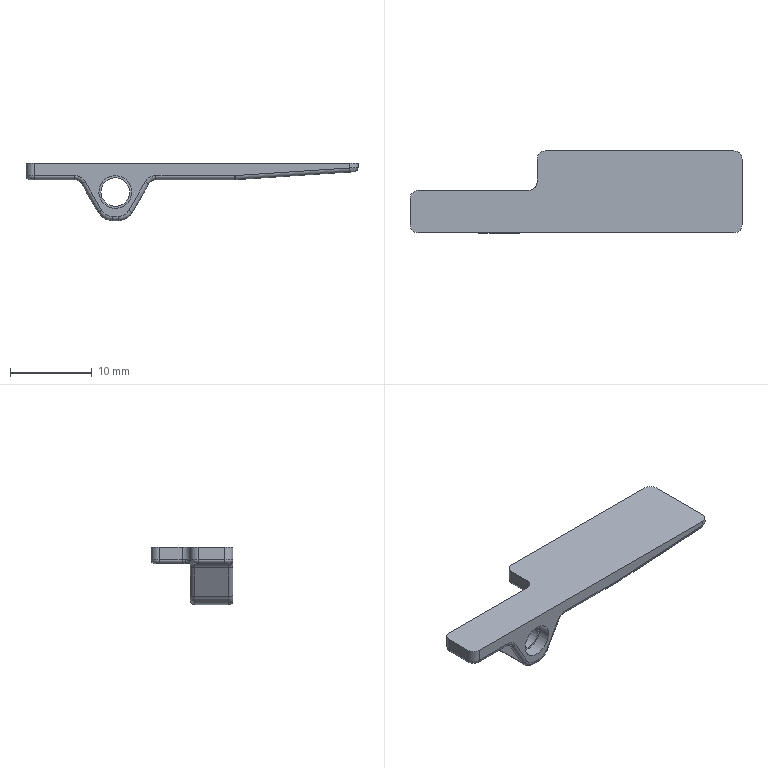NC program | Mastercam | posted with a generic post | part box 40.5 x 10 x 7 mm
Lines 1264 to 2237 of 12178:
(6 FEM |TOOL - 6|DIA. OFF. - 6|LEN. - 6|TOOL DIA. - 6.)
N2590 T6 M6
N2592 G0 G54 G90 X4.981 Y-3.575 C0. B0. S7000 M3
N2594 G43 H6 Z50.
N2596 Z.91
N2598 G1 Z.41 F600.
N2600 G2 X6.981 Y-1.582 Z.3 I2. J-.007 F2000.
N2602 G1 X6.987
N2604 X10.287 Y-1.592 Z.272
N2606 X13.587 Y-1.603 Z.243
N2608 X16.864 Y-1.614 Z.215
N2610 Y-1.212
N2612 Y1.614 Z.191
N2614 X15.161 Z.187
N2616 X11.861 Z.159
N2618 X8.561 Z.13
N2620 X7.761 Z.124
N2622 X5.261 Z.102
N2624 X1.961 Z.074
N2626 X-1.335 Z.046
N2628 G2 X-1.321 Y1.264 I-11.47 J-.649
N2630 G1 X-1.317 Y.965 Z.043
N2632 G2 X-1.596 Y-1.553 Z.021 I-11.488
N2634 G1 X.387 Y-1.56 Z.017
N2636 X3.258 Y-1.569 Z-.007
N2638 X3.687 Y-1.571 Z-.011
N2640 X6.987 Y-1.582 Z-.039
N2642 X10.287 Y-1.592 Z-.067
N2644 X13.587 Y-1.603 Z-.096
N2646 X16.864 Y-1.614 Z-.124
N2648 Y-1.217
N2650 Y1.614 Z-.148
N2652 X15.169 Z-.152
N2654 X11.869 Z-.18
N2656 X8.569 Z-.209
N2658 X7.761 Z-.216
N2660 X5.269 Z-.237
N2662 X1.969 Z-.265
N2664 X-1.335 Z-.293
N2666 G2 X-1.328 Y1.481 I-11.47 J-.649
N2668 X-1.316 Y.965 Z-.298 I-11.477 J-.516
N2670 X-1.596 Y-1.553 Z-.32 I-11.489
N2672 G1 X-.042 Y-1.558 Z-.322
N2674 X3.258 Y-1.569 Z-.35
N2676 X16.864 Y-1.614
N2678 Y1.614
N2680 X7.761
N2682 X-1.335
N2684 G2 X-1.317 Y.965 I-11.47 J-.649
N2686 X-1.596 Y-1.553 I-11.488
N2688 G1 X3.258 Y-1.569
N2690 G2 X3.78 Y-1.992 I-.002 J-.537
N2692 G1 X4.343 Y-4.578
N2694 G3 X4.867 Y-5. I.524 J.114
N2696 G1 X19.151
N2698 G3 X19.235 Y-5.003 I.084 J1.008
N2700 X20.241 Y-4.101 J1.011
N2702 G1 X20.25 Y3.944
N2704 G3 X20.251 Y3.992 I-1.004 J.048
N2706 X19.335 Y4.993 I-1.005
N2708 G1 X7.761 Y5.
N2710 X-4.762
N2712 X-4.721 Y4.463
N2714 X-4.723 Y.245
N2716 G2 X-4.78 Y-.299 I-2.999 J.042
N2718 G1 X-4.829 Y-.528
N2720 G2 X-5.27 Y-1.54 I-2.923 J.674
N2722 G1 X-5.281 Y-1.555
N2724 G2 X-4.75 Y-3.258 I-2.469 J-1.704
N2726 G1 Y-3.944
N2728 G3 X-4.751 Y-3.991 I1.004 J-.047
N2730 X-3.828 Y-4.993 I1.005
N2732 G1 X-3.635 Y-5.
N2734 X4.867
N2736 G3 X5.403 Y-4.464 J.536
N2738 X5.199 Y-4.043 I-.536
N2740 G1 X3.402 Y-2.622
N2742 G2 X3.198 Y-2.201 I.333 J.421
N2744 X3.735 Y-1.665 I.537
N2746 G1 X6.475 Z-.372
N2748 X7.035 Z-.377
N2750 X10.335 Z-.404
N2752 X13.635 Z-.431
N2754 X16.915 Z-.458
N2756 Y-1.302
N2758 Y1.665 Z-.482
N2760 X15.469 Z-.485
N2762 X12.169 Z-.512
N2764 X8.869 Z-.538
N2766 X7.937 Z-.546
N2768 X5.569 Z-.565
N2770 X2.269 Z-.592
N2772 X-1.035 Z-.619
N2774 G2 X-1.028 Y1.509 I-11.533 J-.653
N2776 G1 X-1.02 Y1.261 Z-.621
N2778 X-1.017 Y1.012 Z-.623
N2780 G2 X-1.331 Y-1.665 Z-.645 I-11.551
N2782 G1 X-.125 Z-.646
N2784 X3.175 Z-.673
N2786 X6.475 Z-.7
N2788 X16.915
N2790 Y1.665
N2792 X7.937
N2794 X-1.035
N2796 G2 X-1.017 Y1.012 I-11.533 J-.653
N2798 X-1.331 Y-1.665 I-11.551
N2800 G1 X6.475
N2802 G2 X6.999 Y-2.083 J-.536
N2804 G1 X7.561 Y-4.582
N2806 G3 X8.084 Y-5. I.523 J.118
N2808 G1 X19.151
N2810 G3 X19.235 Y-5.003 I.084 J1.008
N2812 X20.241 Y-4.101 J1.011
N2814 G1 X20.25 Y3.944
N2816 G3 X20.251 Y3.992 I-1.004 J.048
N2818 X19.335 Y4.993 I-1.005
N2820 G1 X7.937 Y5.
N2822 X-4.411
N2824 X-4.371 Y4.511
N2826 Y.383
N2828 X-4.372 Y.252
N2830 G2 X-4.416 Y-.229 I-3. J.035
N2832 X-5.11 Y-1.834 I-3.528 J.571
N2834 X-4.75 Y-3.258 I-2.64 J-1.425
N2836 G1 Y-3.944
N2838 G3 X-4.751 Y-3.991 I1.004 J-.047
N2840 X-3.828 Y-4.993 I1.005
N2842 G1 X-3.635 Y-5.
N2844 X8.084
N2846 G3 X8.62 Y-4.464 J.536
N2848 X8.428 Y-4.052 I-.536
N2850 G1 X6.831 Y-2.72
N2852 G2 X6.638 Y-2.308 I.343 J.412
N2854 X7.174 Y-1.772 I.536
N2856 G1 X9.693 Z-.721
N2858 X10.474 Z-.727
N2860 X13.774 Z-.754
N2862 X17.022 Z-.78
N2864 Y-1.185 Z-.781
N2866 Y1.772 Z-.805
N2868 X15.558 Z-.808
N2870 X12.258 Z-.835
N2872 X8.958 Z-.862
N2874 X8.051 Z-.869
N2876 X5.658 Z-.888
N2878 X2.358 Z-.915
N2880 X-.913 Z-.942
N2882 X-.926 Y1.449
N2884 G2 X-1.24 Y-1.772 Z-.969 I-31.263 J1.417
N2886 G1 X-.207
N2888 X3.093 Z-.996
N2890 X6.393 Z-1.023
N2892 X9.693 Z-1.05
N2894 X17.022
N2896 Y1.772
N2898 X8.051
N2900 X-.913
N2902 G2 X-1.24 Y-1.772 I-31.276 J1.094
N2904 G1 X9.693
N2906 G2 X10.215 Y-2.185 J-.536
N2908 G1 X10.78 Y-4.587
N2910 G3 X11.302 Y-5. I.522 J.123
N2912 G1 X19.151
N2914 G3 X19.235 Y-5.003 I.084 J1.008
N2916 X20.241 Y-4.101 J1.011
N2918 G1 X20.25 Y3.944
N2920 G3 X20.251 Y3.992 I-1.004 J.048
N2922 X19.335 Y4.993 I-1.005
N2924 G1 X8.051 Y5.
N2926 X-4.182
N2928 X-4.142 Y4.48
N2930 Y.353
N2932 X-4.178 Y-.175
N2934 X-4.2 Y-.312
N2936 G2 X-4.386 Y-.983 I-2.964 J.463
N2938 G1 X-4.478 Y-1.193
N2940 G2 X-5.017 Y-2.022 I-3.431 J1.64
N2942 X-4.75 Y-3.258 I-2.733 J-1.237
N2944 G1 Y-3.944
N2946 G3 X-4.751 Y-3.991 I1.004 J-.047
N2948 X-3.828 Y-4.993 I1.005
N2950 G1 X-3.635 Y-5.
N2952 X11.302
N2954 G3 X11.838 Y-4.464 J.536
N2956 X11.66 Y-4.064 I-.536
N2958 G1 X10.252 Y-2.802
N2960 G2 X10.074 Y-2.403 I.358 J.399
N2962 X10.61 Y-1.867 I.536
N2964 G1 X12.91 Z-1.069
N2966 X13.91 Z-1.077
N2968 X17.117 Z-1.103
N2970 Y-1.089 Z-1.104
N2972 Y1.867 Z-1.128
N2974 X15.65 Z-1.131
N2976 X12.35 Z-1.158
N2978 X9.05 Z-1.185
N2980 X8.152 Z-1.192
N2982 X5.75 Z-1.212
N2984 X2.45 Z-1.238
N2986 X-.808 Z-1.265
N2988 X-.816 Y1.391
N2990 G2 X-1.171 Y-1.867 Z-1.292 I-20.708 J.606
N2992 G1 X-.29
N2994 X3.01 Z-1.319
N2996 X6.31 Z-1.346
N2998 X9.61 Z-1.373
N3000 X12.91 Z-1.4
N3002 X17.117
N3004 Y1.867
N3006 X8.152
N3008 X-.808
N3010 G2 X-1.171 Y-1.867 I-20.716 J.13
N3012 G1 X12.91
N3014 G2 X13.431 Y-2.276 J-.536
N3016 G1 X13.998 Y-4.591
N3018 G3 X14.519 Y-5. I.521 J.127
N3020 G1 X19.151
N3022 G3 X19.235 Y-5.003 I.084 J1.008
N3024 X20.241 Y-4.101 J1.011
N3026 G1 X20.25 Y3.944
N3028 G3 X20.251 Y3.992 I-1.004 J.048
N3030 X19.335 Y4.993 I-1.005
N3032 G1 X8.152 Y5.
N3034 X-3.981
N3036 X-3.941 Y4.51
N3038 Y.353
N3040 X-3.98 Y-.191
N3042 X-4.018 Y-.413
N3044 G2 X-4.234 Y-1.1 I-2.949 J.551
N3046 G1 X-4.255 Y-1.147
N3048 G2 X-4.953 Y-2.175 I-3.579 J1.678
N3050 X-4.75 Y-3.258 I-2.797 J-1.084
N3052 G1 Y-3.944
N3054 G3 X-4.751 Y-3.991 I1.004 J-.047
N3056 X-3.828 Y-4.993 I1.005
N3058 G1 X-3.635 Y-5.
N3060 X14.519
N3062 G3 X15.055 Y-4.464 J.536
N3064 X14.892 Y-4.079 I-.536
N3066 G1 X13.628 Y-2.854
N3068 G2 X13.465 Y-2.469 I.374 J.385
N3070 X14.002 Y-1.932 I.537
N3072 G1 X16.128 Z-1.417
N3074 X17.182 Z-1.425
N3076 Y-1.053 Z-1.427
N3078 Y1.932 Z-1.451
N3080 X15.775 Z-1.454
N3082 X12.475 Z-1.481
N3084 X9.175 Z-1.508
N3086 X8.253 Z-1.515
N3088 X5.875 Z-1.535
N3090 X2.575 Z-1.562
N3092 X-.67 Z-1.588
N3094 X-.674 Y1.354
N3096 G2 X-1.06 Y-1.932 Z-1.615 I-17.695 J.415
N3098 G1 X-.372
N3100 X2.928 Z-1.642
N3102 X6.228 Z-1.669
N3104 X9.528 Z-1.696
N3106 X12.828 Z-1.723
N3108 X16.128 Z-1.75
N3110 X17.182
N3112 Y1.932
N3114 X8.253
N3116 X-.67
N3118 G2 X-.669 Y1.769 I-17.699 J-.163
N3120 X-1.06 Y-1.932 I-17.7
N3122 G1 X16.128
N3124 G2 X16.648 Y-2.337 J-.537
N3126 G1 X17.217 Y-4.595
N3128 G3 X17.737 Y-5. I.52 J.131
N3130 G1 X19.151
N3132 G3 X19.235 Y-5.003 I.084 J1.008
N3134 X20.241 Y-4.101 J1.011
N3136 G1 X20.25 Y3.944
N3138 G3 X20.251 Y3.992 I-1.004 J.048
N3140 X19.335 Y4.993 I-1.005
N3142 G1 X8.253 Y5.
N3144 X-3.778
N3146 X-3.737 Y4.489
N3148 Y.383
N3150 X-3.739 Y.257
N3152 G2 X-3.78 Y-.213 I-2.999 J.03
N3154 G1 X-3.822 Y-.444
N3156 G2 X-4.035 Y-1.11 I-2.944 J.576
N3158 G1 X-4.172 Y-1.385
N3160 G2 X-4.9 Y-2.323 I-3.557 J2.01
N3162 X-4.75 Y-3.258 I-2.85 J-.936
N3164 G1 Y-3.944
N3166 G3 X-4.751 Y-3.991 I1.004 J-.047
N3168 X-3.828 Y-4.993 I1.005
N3170 G1 X-3.635 Y-5.
N3172 X17.737
N3174 G3 X18.273 Y-4.464 J.536
N3176 X17.861 Y-3.942 I-.536
N3178 G1 X13.866 Y-2.99
N3180 G2 X13.455 Y-2.469 I.125 J.521
N3182 X13.991 Y-1.932 I.536
N3184 G1 X17.182 Z-1.776
N3186 Y-1.094 Z-1.777
N3188 Y-.324 Z-1.783
N3190 Y1.932 Z-1.801
N3192 X15.867 Z-1.804
N3194 X12.567 Z-1.831
N3196 X9.267 Z-1.858
N3198 X8.354 Z-1.865
N3200 X5.967 Z-1.885
N3202 X2.667 Z-1.912
N3204 X-.468 Z-1.937
N3206 X-.471 Y1.446 Z-1.938
N3208 X-.487 Y.96
N3210 G2 X-.86 Y-1.932 Z-1.962 I-17.931 J.84
N3212 G1 X1.101 Z-1.965
N3214 X4.401 Z-1.992
N3216 X7.701 Z-2.019
N3218 X11.001 Z-2.046
N3220 X14.301 Z-2.073
N3222 X17.182 Z-2.097
N3224 Y-.324 Z-2.1
N3226 Y1.932
N3228 X8.354
N3230 X-.468
N3232 Y1.8
N3234 G2 X-.86 Y-1.932 I-17.95
N3236 G1 X17.182
N3238 Y-.324
N3240 G2 X17.588 Y.196 I.537
N3242 G1 X19.841 Y.762
N3244 G3 X20.247 Y1.282 I-.13 J.52
N3246 G1 X20.25 Y3.944
N3248 G3 X20.251 Y3.992 I-1.004 J.048
N3250 X19.335 Y4.993 I-1.005
N3252 G1 X8.354 Y5.
N3254 X-3.576
N3256 X-3.536 Y4.51
N3258 X-3.535 Y.383
N3260 X-3.536 Y.256
N3262 G2 X-3.582 Y-.234 I-3. J.031
N3264 X-4.858 Y-2.462 I-3.562 J.561
N3266 X-4.742 Y-3.629 I-5.802 J-1.167
N3268 X-4.75 Y-3.944 I-5.918
N3270 G3 X-4.751 Y-3.991 I1.004 J-.047
N3272 X-3.828 Y-4.993 I1.005
N3274 G1 X-3.635 Y-5.
N3276 X19.151
N3278 G3 X19.235 Y-5.003 I.084 J1.008
N3280 X20.241 Y-4.101 J1.011
N3282 G1 X20.247 Y1.282
N3284 G3 X19.711 Y1.818 I-.536
N3286 X19.204 Y1.457 J-.536
N3288 G1 X18.227 Y-1.37
N3290 G2 X17.72 Y-1.731 I-.507 J.175
N3292 X17.184 Y-1.195 J.536
N3294 G1 Y1.934 Z-2.126
N3296 X16.228 Z-2.127
N3298 X16.137
N3300 X12.837 Z-2.154
N3302 X9.537 Z-2.181
N3304 X8.455 Z-2.19
N3306 X6.237 Z-2.208
N3308 X2.937 Z-2.235
N3310 X-.268 Z-2.261
N3312 X-.27 Y1.566
N3314 X-.28 Y1.197 Z-2.262
N3316 G2 X-.659 Y-1.934 Z-2.287 I-18.716 J.68
N3318 G1 X.762 Z-2.288
N3320 X4.062 Z-2.315
N3322 X7.362 Z-2.342
N3324 X10.662 Z-2.369
N3326 X13.962 Z-2.396
N3328 X17.184 Z-2.422
N3330 Y-1.224 Z-2.423
N3332 Y1.934 Z-2.449
N3334 X16.228 Z-2.45
N3336 X8.455
N3338 X-.268
N3340 Y1.877
N3342 G2 X-.659 Y-1.934 I-18.728
N3344 G1 X17.184
N3346 Y1.934
N3348 X16.228
N3350 G2 X15.708 Y2.34 J.537
N3352 G1 X15.141 Y4.591
N3354 G3 X14.621 Y4.996 I-.52 J-.131
N3356 G1 X8.455 Y5.
N3358 X-3.374
N3360 X-3.333 Y4.499
N3362 Y.383
N3364 X-3.334 Y.256
N3366 G2 X-3.384 Y-.255 I-3. J.031
N3368 G1 X-3.434 Y-.51
N3370 G2 X-3.635 Y-1.121 I-2.934 J.627
N3372 G1 X-3.651 Y-1.155
N3374 X-3.869 Y-1.556
N3376 X-4.149 Y-1.95
N3378 X-4.305 Y-2.131
N3380 G2 X-4.826 Y-2.588 I-2.227 J2.01
N3382 X-4.743 Y-3.642 I-6.674 J-1.054
N3384 X-4.75 Y-3.944 I-6.757
N3386 G3 X-4.751 Y-3.991 I1.004 J-.047
N3388 X-3.828 Y-4.993 I1.005
N3390 G1 X-3.635 Y-5.
N3392 X19.151
N3394 G3 X19.235 Y-5.003 I.084 J1.008
N3396 X20.241 Y-4.101 J1.011
N3398 G1 X20.25 Y3.944
N3400 G3 X20.251 Y3.992 I-1.004 J.048
N3402 X19.335 Y4.993 I-1.005
N3404 G1 X14.621 Y4.996
N3406 G3 X14.085 Y4.46 J-.536
N3408 X14.394 Y3.974 I.536
N3410 G1 X16.579 Y2.955
N3412 G2 X16.888 Y2.469 I-.227 J-.486
N3414 X16.352 Y1.933 I-.536
N3416 G1 X13.052 Z-2.477
N3418 X13.012
N3420 X9.752 Z-2.504
N3422 X8.556 Z-2.514
N3424 X6.452 Z-2.531
N3426 X3.152 Z-2.558
N3428 X-.064 Z-2.584
N3430 X-.068 Y1.597
N3432 X-.078 Y1.261 Z-2.585
N3434 G2 X-.458 Y-1.933 Z-2.611 I-20.024 J.76
N3436 G1 X.754 Z-2.612
N3438 X4.054 Z-2.638
N3440 X7.354 Z-2.665
N3442 X10.654 Z-2.692
N3444 X13.954 Z-2.719
N3446 X17.183 Z-2.746
N3448 Y-1.25
N3450 Y1.933 Z-2.772
N3452 X16.312 Z-2.773
N3454 X13.012 Z-2.8
N3456 X8.556
N3458 X-.064
N3460 G2 X-.458 Y-1.933 I-20.038 J.088
N3462 G1 X17.183
N3464 Y1.933
N3466 X13.012
N3468 G2 X12.492 Y2.338 J.536
N3470 G1 X11.925 Y4.593
N3472 G3 X11.406 Y4.998 I-.52 J-.131
N3474 G1 X8.556 Y5.
N3476 X-3.172
N3478 X-3.132 Y4.51
N3480 X-3.131 Y.383
N3482 X-3.132 Y.256
N3484 G2 X-3.195 Y-.324 I-3. J.031
N3486 G1 X-3.226 Y-.48
N3488 X-3.361 Y-.941
N3490 G2 X-3.67 Y-1.561 I-2.821 J1.021
N3492 X-4.802 Y-2.705 I-2.987 J1.821
N3494 X-4.746 Y-3.669 I-8.235 J-.964
N3496 X-4.75 Y-3.944 I-8.291
N3498 G3 X-4.751 Y-3.991 I1.004 J-.047
N3500 X-3.828 Y-4.993 I1.005
N3502 G1 X-3.635 Y-5.
N3504 X19.151
N3506 G3 X19.235 Y-5.003 I.084 J1.008
N3508 X20.241 Y-4.101 J1.011
N3510 G1 X20.25 Y3.944
N3512 G3 X20.251 Y3.992 I-1.004 J.048
N3514 X19.335 Y4.993 I-1.005
N3516 G1 X11.406 Y4.998
N3518 X11.405
N3520 G3 X10.869 Y4.462 J-.536
N3522 X11.189 Y3.971 I.536
N3524 G1 X13.475 Y2.961
N3526 G2 X13.794 Y2.471 I-.217 J-.49
N3528 X13.258 Y1.935 I-.536
N3530 G1 X9.958 Z-2.827
N3532 X9.797 Z-2.828
N3534 X8.657 Z-2.838
N3536 X6.658 Z-2.854
N3538 X3.358 Z-2.881
N3540 X.136 Z-2.907
N3542 X.119 Y1.304 Z-2.908
N3544 G2 X-.256 Y-1.935 Z-2.934 I-22.012 J.91
N3546 G1 X.752 Z-2.935
N3548 X4.052 Z-2.962
N3550 X7.352 Z-2.988
N3552 X10.652 Z-3.015
N3554 X13.952 Z-3.042
N3556 X17.185 Z-3.069
N3558 Y-1.27
N3560 Y1.935 Z-3.095
N3562 X16.397 Z-3.096
N3564 X13.097 Z-3.123
N3566 X9.797 Z-3.15
N3568 X8.657
N3570 X.136
N3572 G2 X-.256 Y-1.935 I-22.029 J.279
N3574 G1 X17.185
N3576 Y1.935
N3578 X9.797
N3580 G2 X9.261 Y2.453 J.536
N3582 G1 X9.193 Y4.482
N3584 G3 X8.657 Y5. I-.536 J-.018
N3586 G1 X-2.97
N3588 X-2.93 Y4.535
N3590 X-2.929 Y.383
N3592 X-2.93 Y.255
N3594 G2 X-2.998 Y-.346 I-3. J.032
N3596 G1 X-3.041 Y-.551
N3598 G2 X-3.252 Y-1.17 I-2.928 J.655
N3600 G1 X-3.271 Y-1.21
N3602 G2 X-3.567 Y-1.708 I-2.717 J1.273
N3604 G1 X-3.571 Y-1.715
N3606 G2 X-3.999 Y-2.233 I-11.144 J8.774
N3608 X-4.562 Y-2.681 I-2.138 J2.104
N3610 G1 X-4.783 Y-2.815
N3612 G2 X-4.748 Y-3.746 I-12.496 J-.931
N3614 X-4.75 Y-3.944 I-12.531
N3616 G3 X-4.751 Y-3.991 I1.004 J-.047
N3618 X-3.828 Y-4.993 I1.005
N3620 G1 X-3.635 Y-5.
N3622 X19.151
N3624 G3 X19.235 Y-5.003 I.084 J1.008
N3626 X20.241 Y-4.101 J1.011
N3628 G1 X20.25 Y3.944
N3630 G3 X20.251 Y3.992 I-1.004 J.048
N3632 X19.335 Y4.993 I-1.005
N3634 G1 X8.657 Y5.
N3636 G3 X8.121 Y4.464 J-.536
N3638 X8.41 Y3.988 I.536
N3640 G1 X10.416 Y2.946
N3642 G2 X10.705 Y2.47 I-.248 J-.476
N3644 X10.168 Y1.934 I-.537
N3646 G1 X8.758 Z-3.162
N3648 X7.049 Z-3.175
N3650 X6.868 Z-3.177
N3652 X3.568 Z-3.204
N3654 X.339 Z-3.23
N3656 X.322 Y1.34 Z-3.231
N3658 G2 X-.056 Y-1.934 Z-3.258 I-22.233 J.907
N3660 G1 X.735
N3662 X4.035 Z-3.285
N3664 X7.335 Z-3.312
N3666 X10.635 Z-3.338
N3668 X13.935 Z-3.365
N3670 X17.184 Z-3.392
N3672 Y-1.358
N3674 Y1.934 Z-3.419
N3676 X16.949
N3678 X13.649 Z-3.446
N3680 X10.349 Z-3.473
N3682 X8.758 Z-3.486
N3684 X7.049 Z-3.5
N3686 X.339
N3688 G2 X-.056 Y-1.934 I-22.25 J.313
N3690 G1 X17.184
N3692 Y1.934
N3694 X8.758
N3696 X7.049
N3698 G2 X6.529 Y2.339 J.536
N3700 G1 X5.96 Y4.595
N3702 G3 X5.44 Y5. I-.52 J-.131
N3704 G1 X-2.768
N3706 X-2.728 Y4.51
N3708 Y.255
N3710 G2 X-2.793 Y-.334 I-3. J.032
N3712 G1 X-2.826 Y-.49
N3714 X-2.924 Y-.847
N3716 G2 X-3.302 Y-1.618 I-2.855 J.921
N3718 G1 X-3.502 Y-1.896
N3720 X-3.839 Y-2.275
N3722 G2 X-4.769 Y-2.918 I-3.227 J3.671
N3724 X-4.75 Y-3.944 I-136.234 J-3.104
N3726 G3 X-4.751 Y-3.991 I1.004 J-.047
N3728 X-3.828 Y-4.993 I1.005
N3730 G1 X-3.635 Y-5.
N3732 X19.151
N3734 G3 X19.235 Y-5.003 I.084 J1.008
N3736 X20.241 Y-4.101 J1.011
N3738 G1 X20.25 Y3.944
N3740 G3 X20.251 Y3.992 I-1.004 J.048
N3742 X19.335 Y4.993 I-1.005
N3744 G1 X8.758 Y5.
N3746 X5.44
N3748 G3 X4.904 Y4.464 J-.536
N3750 X5.208 Y3.98 I.536
N3752 G1 X7.344 Y2.954
N3754 G2 X7.649 Y2.47 I-.232 J-.484
N3756 X7.112 Y1.934 I-.537
N3758 G1 X3.831 Z-3.527
N3760 X3.812
N3762 X.541 Z-3.554
N3764 X.555 Y1.648
N3766 X.562 Y1.361
N3768 X.563 Y1.204 Z-3.555
N3770 G2 X.148 Y-1.934 Z-3.581 I-12.08
N3772 G1 X.734
N3774 X4.034 Z-3.608
N3776 X7.334 Z-3.635
N3778 X10.634 Z-3.662
N3780 X13.934 Z-3.688
N3782 X17.184 Z-3.715
N3784 Y-1.362
N3786 Y1.934 Z-3.742
N3788 X17.031
N3790 X13.731 Z-3.769
N3792 X10.431 Z-3.796
N3794 X8.859 Z-3.809
N3796 X7.131 Z-3.823
N3798 X3.831 Z-3.85
N3800 X.541
N3802 G2 X.563 Y1.204 I-12.058 J-.73
N3804 X.148 Y-1.934 I-12.08
N3806 G1 X17.184
N3808 Y1.934
N3810 X8.859
N3812 X3.831
N3814 G2 X3.311 Y2.339 J.536
N3816 G1 X2.742 Y4.595
N3818 G3 X2.222 Y5. I-.52 J-.131
N3820 G1 X-2.566
N3822 X-2.525 Y4.493
N3824 X-2.526 Y.255
N3826 G2 X-2.592 Y-.34 I-3. J.032
N3828 G1 X-2.647 Y-.585
N3830 G2 X-4.761 Y-3.007 I-3.496 J.918
N3832 G1 X-4.75 Y-3.944
N3834 G3 X-4.751 Y-3.991 I1.004 J-.047
N3836 X-3.828 Y-4.993 I1.005
N3838 G1 X-3.635 Y-5.
N3840 X19.151
N3842 G3 X19.235 Y-5.003 I.084 J1.008
N3844 X20.241 Y-4.101 J1.011
N3846 G1 X20.25 Y3.944
N3848 G3 X20.251 Y3.992 I-1.004 J.048
N3850 X19.335 Y4.993 I-1.005
N3852 G1 X8.859 Y5.
N3854 X2.222
N3856 G3 X1.686 Y4.464 J-.536
N3858 X2.12 Y3.937 I.536
N3860 G1 X6.955 Y2.996
N3862 G2 X7.389 Y2.469 I-.103 J-.527
N3864 X6.852 Y1.933 I-.537
N3866 G1 X3.552 Z-3.877
N3868 X.744 Z-3.9
N3870 G2 X.751 Y1.803 I-11.841 J-.748
N3872 G1 X.765 Y1.409 Z-3.901
N3874 X.766 Y1.014 Z-3.902
N3876 X.754 Y.619 Z-3.903
N3878 X.728 Y.225 Z-3.904
N3880 G2 X.35 Y-1.933 Z-3.922 I-11.825 J.96
N3882 G1 X3.225 Z-3.931
N3884 X6.525 Z-3.958
N3886 X9.825 Z-3.985
N3888 X13.125 Z-4.012
N3890 X16.425 Z-4.038
N3892 X17.183 Z-4.045
N3894 Y1.279 Z-4.065
N3896 Y1.933 Z-4.071
N3898 X13.949 Z-4.092
N3900 X10.649 Z-4.119
N3902 X8.96 Z-4.133
N3904 X7.349 Z-4.146
N3906 X4.049 Z-4.173
N3908 X.744 Z-4.2
N3910 G2 X.751 Y1.803 I-11.841 J-.748
N3912 X.767 Y1.185 I-11.848 J-.618
N3914 X.35 Y-1.933 I-11.864
N3916 G1 X17.183
N3918 Y1.933
N3920 X8.96
N3922 X.744
N3924 G2 X.751 Y1.803 I-11.841 J-.748
N3926 X.752 Y1.775 I-.535 J-.028
N3928 X.348 Y1.256 I-.536
N3930 G1 X-1.926 Y.674
N3932 G3 X-2.328 Y.195 I.132 J-.519
N3934 G2 X-2.477 Y-.703 I-5.119 J.387
N3936 G1 X-2.495 Y-.764
N3938 G2 X-2.963 Y-1.713 I-2.882 J.832
N3940 G1 X-3.189 Y-2.008
N3942 G2 X-4.755 Y-3.082 I-2.805 J2.409
N3944 G1 X-4.75 Y-3.944
N3946 G3 X-4.751 Y-3.991 I1.004 J-.047
N3948 X-3.828 Y-4.993 I1.005
N3950 G1 X-3.635 Y-5.
N3952 X19.151
N3954 G3 X19.235 Y-5.003 I.084 J1.008
N3956 X20.241 Y-4.101 J1.011
N3958 G1 X20.25 Y3.944
N3960 G3 X20.251 Y3.992 I-1.004 J.048
N3962 X19.335 Y4.993 I-1.005
N3964 G1 X8.96 Y5.
N3966 X-2.363
N3968 X-2.323 Y4.51
N3970 X-2.324 Y.254
N3972 G2 X-2.328 Y.195 I-5.123 J.328
N3974 G3 X-2.329 Y.155 I.534 J-.04
N3976 X-1.794 Y-.38 I.535
N3978 X-1.684 Y-.37 J.535
N3980 G1 X4.289 Y.87
N3982 G3 X4.717 Y1.396 I-.109 J.526
N3984 X4.18 Y1.932 I-.537
N3986 G1 X.959 Z-4.226
N3988 X.962 Y1.576 Z-4.227
N3990 X.957 Y1.22
N3992 G2 X.607 Y-1.747 Z-4.251 I-16.039 J.392
N3994 G1 X.566 Y-1.932 Z-4.252
N3996 X1.935 Z-4.254
N3998 X5.235 Z-4.281
N4000 X8.535 Z-4.308
N4002 X11.835 Z-4.335
N4004 X15.135 Z-4.362
N4006 X17.182 Z-4.378
N4008 Y.657 Z-4.388
N4010 Y1.932 Z-4.399
N4012 X14.138 Z-4.415
N4014 X10.838 Z-4.442
N4016 X9.067 Z-4.457
N4018 X7.538 Z-4.469
N4020 X4.238 Z-4.496
N4022 X.959 Z-4.523
N4024 X.962 Y1.534
N4026 G2 X.607 Y-1.747 Z-4.55 I-16.044 J.078
N4028 X.566 Y-1.932 I-15.689 J3.359
N4030 G1 X17.182
N4032 Y1.932
N4034 X9.067
N4036 X.959
N4038 G2 X.962 Y1.612 I-16.041 J-.32
N4040 X.607 Y-1.747 I-16.044
N4042 X.082 Y-2.172 I-.525 J.112
N4044 X.049 Y-2.17 J.537
N4046 G1 X-2.703 Y-2.
N4048 G3 X-2.736 Y-1.999 I-.033 J-.535
N4050 X-3.119 Y-2.161 J-.536
N4052 G2 X-4.752 Y-3.147 I-2.718 J2.655
N4054 G1 X-4.75 Y-3.944
N4056 G3 X-4.751 Y-3.991 I1.004 J-.047
N4058 X-3.828 Y-4.993 I1.005
N4060 G1 X-3.635 Y-5.
N4062 X19.151
N4064 G3 X19.235 Y-5.003 I.084 J1.008
N4066 X20.241 Y-4.101 J1.011
N4068 G1 X20.25 Y3.944
N4070 G3 X20.251 Y3.992 I-1.004 J.048
N4072 X19.335 Y4.993 I-1.005
N4074 G1 X9.067 Y5.
N4076 X-2.151
N4078 X-2.11 Y4.498
N4080 Y.284
N4082 G2 X-2.272 Y-.741 I-4.046 J.113
N4084 G1 X-2.312 Y-.865
N4086 G2 X-2.631 Y-1.54 I-2.851 J.933
N4088 X-3.1 Y-2.141 I-4.862 J3.315
N4090 X-3.119 Y-2.161 I-2.737 J2.635
N4092 G3 X-3.271 Y-2.535 I.383 J-.374
N4094 X-2.736 Y-3.07 I.535
N4096 G1 X-2.641 Y-3.062
N4098 X-2.549 Y-3.037
N4100 X7.841 Y.827
N4102 G3 X8.19 Y1.329 I-.187 J.502
N4104 X7.654 Y1.866 I-.536
N4106 G1 X4.354 Z-4.577
N4108 X1.684 Z-4.599
N4110 X1.577 Y.082 Z-4.604
N4112 X1.461 Y-1.866 Z-4.62
N4114 X3.069 Z-4.624
N4116 X4.241 Z-4.631
N4118 X7.541 Z-4.658
N4120 X10.841 Z-4.685
N4122 X14.141 Z-4.712
N4124 X17.115 Z-4.736
N4126 Y-.436 Z-4.738
N4128 Y1.866 Z-4.757
N4130 X14.751 Z-4.765
N4132 X11.451 Z-4.792
N4134 X9.391 Z-4.809
N4136 X8.151 Z-4.819
N4138 X4.851 Z-4.846
N4140 X1.684 Z-4.872
N4142 X1.639 Y1.108 Z-4.873
N4144 X1.461 Y-1.866 Z-4.897
N4146 X3.069 Z-4.9
N4148 X17.115
N4150 Y1.866
N4152 X9.391
N4154 X1.684
N4156 X1.461 Y-1.866
N4158 X3.069
N4160 G2 X3.59 Y-2.274 J-.536
N4162 G1 X4.157 Y-4.591
N4164 G3 X4.678 Y-5. I.521 J.127
N4166 G1 X19.151
N4168 G3 X19.235 Y-5.003 I.084 J1.008
N4170 X20.241 Y-4.101 J1.011
N4172 G1 X20.25 Y3.944
N4174 G3 X20.251 Y3.992 I-1.004 J.048
N4176 X19.335 Y4.993 I-1.005
N4178 G1 X9.391 Y5.
N4180 X-1.487
N4182 G2 X-1.424 Y3.832 I-10.815 J-1.168
N4184 G1 Y3.77
N4186 X-1.471 Y-.329
N4188 G2 X-1.569 Y-1.062 I-3. J.028
N4190 G1 X-1.583 Y-1.113
N4192 G2 X-3.817 Y-3.278 I-2.902 J.76
N4194 X-4.579 Y-3.376 I-.762 J2.902
N4196 X-4.75 Y-3.371 J3.
N4198 G1 Y-3.944
N4200 G3 X-4.751 Y-3.991 I1.004 J-.047
N4202 X-3.828 Y-4.993 I1.005
N4204 G1 X-3.635 Y-5.
N4206 X4.678
N4208 G3 X4.8 Y-4.986 J.536
N4210 G1 X19.836 Y-1.46
N4212 G3 X20.25 Y-.938 I-.122 J.522
N4214 G1 Y2.362 Z-4.929
N4216 Y3.944 Z-4.943
N4218 G3 X20.251 Y3.992 I-1.004 J.048
N4220 X19.335 Y4.993 Z-4.953 I-1.005
N4222 G1 X18.259 Y4.994 Z-4.958
N4224 X14.959 Y4.997 Z-4.986
N4226 X11.665 Y5. Z-5.015
N4228 X11.708 Y4.448
N4230 Y4.431
N4232 Y1.131 Z-5.044
N4234 Y0. Z-5.054
N4236 Y-2.169 Z-5.073
N4238 Y-4.447 Z-5.093
N4240 X11.665 Y-5. Z-5.097
N4242 X13.403 Z-5.102
N4244 X16.703 Z-5.13
N4246 G3 X17.239 Y-4.464 J.536
N4248 X17.178 Y-4.215 I-.536
N4250 G1 X16.227 Y-2.399
N4252 G2 X16.166 Y-2.15 I.476 J.249
N4254 X16.703 Y-1.614 I.537
N4256 G1 X16.864
N4258 Y1.614
N4260 X15.094
N4262 Y0.
N4264 Y-1.614
N4266 X16.703
N4268 G2 X17.226 Y-2.035 J-.536
N4270 G1 X17.788 Y-4.579
N4272 G3 X18.311 Y-5. I.523 J.115
N4274 G1 X19.151
N4276 G3 X19.235 Y-5.003 I.084 J1.008
N4278 X20.241 Y-4.101 J1.011
N4280 G1 X20.25 Y-3.944
N4282 Y3.944
N4284 G3 X20.251 Y3.992 I-1.004 J.048
N4286 X19.335 Y4.993 I-1.005
N4288 G1 X11.665 Y5.
N4290 X11.708 Y4.448
N4292 Y0.
N4294 Y-4.447
N4296 X11.665 Y-5.
N4298 X18.311
N4300 G3 X18.847 Y-4.464 J.536
N4302 X18.748 Y-4.153 I-.536
N4304 G1 X14.472 Y1.854
N4306 G3 X14.035 Y2.079 I-.437 J-.311
N4308 X13.499 Y1.543 J-.536
N4310 G1 Y-1.757 Z-5.154
N4312 Y-4.463 Z-5.174
N4314 X13.452 Y-5. Z-5.178
N4316 X14.112
N4318 X17.412 Z-5.202
N4320 X19.151 Z-5.215
N4322 G3 X19.234 Y-5.003 I.083 J1.012
N4324 X20.225 Y-4.207 Z-5.223 J1.015
N4326 G1 X20.25 Y-3.944 Z-5.224
N4328 Y-3.316 Z-5.226
N4330 Y-.016 Z-5.25
N4332 G3 X19.714 Y.52 I-.536
N4334 X19.464 Y.459 J-.536
N4336 G1 X17.661 Y-.491
N4338 G2 X17.411 Y-.553 I-.25 J.475
N4340 X16.875 Y-.016 J.537
N4342 G1 Y0.
N4344 Y1.625
N4346 X16.874
N4348 Y-1.625
N4350 X16.875
N4352 Y-.016
N4354 G2 X17.411 Y.52 I.536
N4356 X17.657 Y.46 J-.536
N4358 G1 X19.467 Y-.476
N4360 G3 X19.714 Y-.536 I.247 J.476
N4362 X20.25 Y0. J.536
N4364 G1 Y3.944
N4366 X20.225 Y4.207
N4368 G3 X19.444 Y4.978 I-.976 J-.208
N4370 G1 X19.151 Y5.
N4372 X13.452
N4374 X13.499 Y4.463
N4376 Y-4.463
N4378 X13.452 Y-5.
N4380 X19.151
N4382 G3 X19.234 Y-5.003 I.083 J1.012
N4384 X20.225 Y-4.207 J1.015
N4386 G1 X20.25 Y-3.944
N4388 Y0.
N4390 G3 X19.714 Y.536 I-.536
N4392 X19.239 Y.249 J-.536
N4394 G1 X16.895 Y-4.214
N4396 G3 X16.833 Y-4.464 I.475 J-.25
N4398 X17.37 Y-5. I.537
N4400 G1 X19.151 Z-5.264
N4402 X19.234 Y-5.003 Z-5.265
N4404 G3 X20.225 Y-4.207 Z-5.273 J1.015
N4406 G1 X20.25 Y-3.944 Z-5.274
N4408 Y-3.389 Z-5.276
N4410 Y-.089 Z-5.302
N4412 Y0.
N4414 Y1.609 Z-5.315
N4416 Y3.211 Z-5.327
N4418 Y3.944 Z-5.333
N4420 X20.225 Y4.207 Z-5.335
N4422 G3 X19.335 Y4.993 Z-5.343 I-.974 J-.206
N4424 G1 X16.936 Y5. Z-5.353
N4426 X16.98 Y4.46
N4428 Y3.659
N4430 Y.359 Z-5.379
N4432 Y-2.941 Z-5.405
N4434 Y-4.461 Z-5.416
N4436 X16.936 Y-5. Z-5.421
N4438 X19.151 Z-5.428
N4440 X19.269 Y-5.003
N4442 X19.387 Y-4.992 Z-5.429
N4444 X19.502 Y-4.967 Z-5.43
N4446 X19.614 Y-4.929
N4448 G3 X20.225 Y-4.207 Z-5.438 I-.38 J.941
N4450 G1 X20.25 Y-3.944 Z-5.439
N4452 Y-1.691 Z-5.456
N4454 Y0. Z-5.469
N4456 Y1.609 Z-5.482
N4458 Y3.944
N4460 X20.225 Y4.207
N4462 G3 X19.335 Y4.993 I-.974 J-.206
N4464 G1 X16.936 Y5.
N4466 X16.98 Y4.46
N4468 Y-4.461
N4470 X16.936 Y-5.
N4472 X19.151
N4474 G3 X19.234 Y-5.003 I.083 J1.012
N4476 X20.225 Y-4.207 J1.015
N4478 G1 X20.25 Y-3.944
N4480 Y0.
N4482 Y1.609
N4484 G3 X19.714 Y2.145 I-.536
N4486 X19.177 Y1.609 J-.536
N4488 G1 Y-.083
N4490 G3 X19.714 Y-.619 I.537
N4492 X20.25 Y-.083 J.536
N4494 G1 Y0.
N4496 Y3.217 Z-5.505
N4498 Y3.944
N4500 X20.225 Y4.207
N4502 G3 X19.335 Y4.993 I-.974 J-.206
N4504 G1 X18.707 Y5.
N4506 G2 X18.753 Y4.473 I-2.954 J-.527
N4508 G1 Y2.859
N4510 Y-.441 Z-5.529
N4512 Y-4.471 Z-5.553
N4514 G2 X18.706 Y-5. I-3.
N4516 G1 X19.151
N4518 G3 X19.234 Y-5.003 I.083 J1.012
N4520 X20.225 Y-4.207 J1.015
N4522 G1 X20.25 Y-3.944
N4524 Y-3.382
N4526 Y-.083 Z-5.576
N4528 Y0. Z-5.577
N4530 Y3.217 Z-5.6
N4532 Y3.944
N4534 X20.225 Y4.207